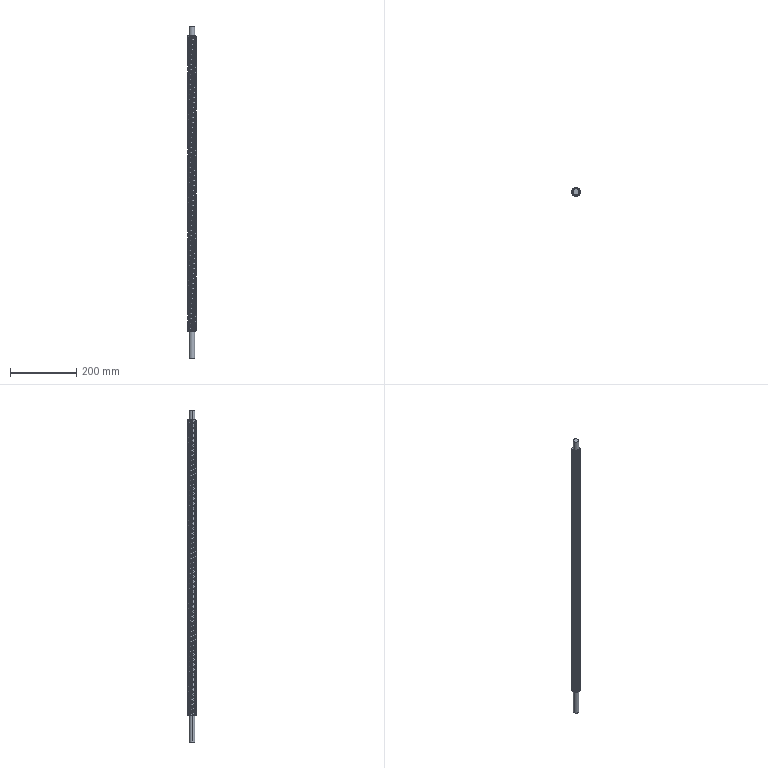Part | SolidWorks | features BaseBody 1 | 1 solid | 380 faces | box 25 x 25 x 1000 mm | volume 414635 mm3 | cylinder 362 | spline 14 | plane 4 | commonest cylinder face diameters 25 x358 17 x4